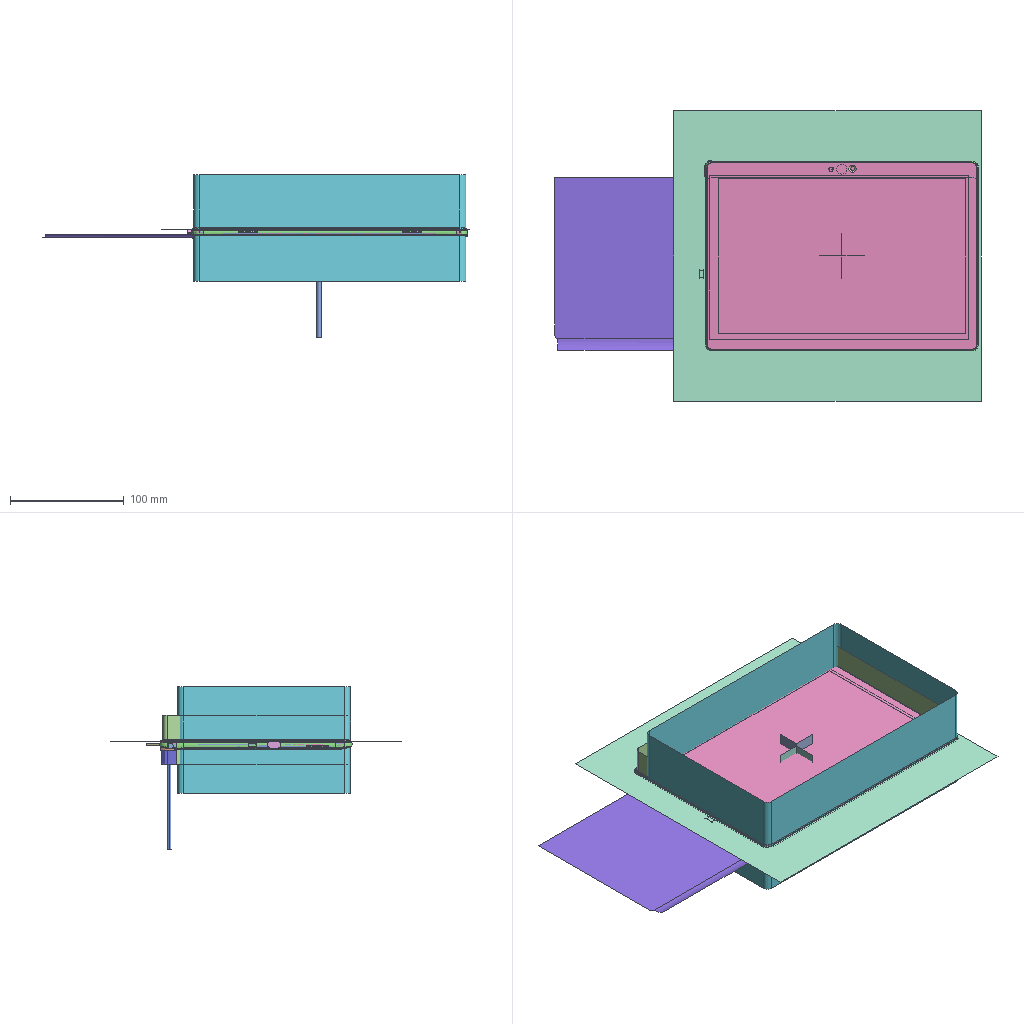Assembly | Creo | 321 different items | 1427 placed | box 375 x 255 x 143 mm
Parts list (item | name | quantity | parent item | size | volume):
1 | - | x1 | in 286 | 3.033 x 2.65 x 3.533 mm | 2.841 mm3
2 | - | x1 | in 314 | 0.2016 x 0.1 x 0.1125 mm | 0.002268 mm3
3 | - | x1 | in 314 | 0.2016 x 0.1 x 0.1125 mm | 0.002268 mm3
4 | - | x1 | in 314 | 0.2016 x 0.1 x 0.1125 mm | 0.002268 mm3
5 | - | x1 | in 314 | 0.2016 x 0.1 x 0.1125 mm | 0.002268 mm3
6 | - | x1 | in 314 | 0.2016 x 0.1 x 0.1125 mm | 0.002268 mm3
7 | - | x1 | in 314 | 0.2016 x 0.1 x 0.1125 mm | 0.002268 mm3
8 | - | x1 | in 314 | 0.2016 x 0.1 x 0.1125 mm | 0.002268 mm3
9 | - | x1 | in 314 | 0.2016 x 0.1 x 0.1125 mm | 0.002268 mm3
10 | - | x1 | in 314 | 0.2016 x 0.1 x 0.1125 mm | 0.002268 mm3
11 | - | x1 | in 314 | 0.2016 x 0.1 x 0.1125 mm | 0.002268 mm3
12 | - | x1 | in 286 | 3.115 x 3.9 x 2.85 mm | 3.729 mm3
13 | - | x14 | in 314 | 1.218 x 0.6006 x 0.55 mm | 0.4024 mm3
14 | - | x1 | in 304 | 0.365 x 0.3 x 0.5 mm | 0.03234 mm3
15 | - | x1 | in 306 | 0.12 x 0.73 x 2.69 mm | 0.132 mm3
16 | - | x1 | in 306 | 0.365 x 0.3 x 0.5 mm | 0.03234 mm3
17 | - | x1 | in 304 | 0.12 x 0.73 x 2.69 mm | 0.132 mm3
18 | - | x1 | in 314 | 1.75 x 2.2 x 1.1 mm | 4.235 mm3
19 | - | x3 | in 314 | 2 x 1.625 x 1.1 mm | 3.576 mm3
20 | - | x1 | in 308 | 42 x 1.4 x 3.75 mm | 72.804 mm3
21 | - | x1 | in 293 | 228.88 x 4.8 x 3.7 mm | 376.003 mm3
22 | - | x1 | in 293 | 8 x 8 x 0.5 mm | 23.747 mm3
23 | - | x1 | in 286 | 3.115 x 3.9 x 2.95 mm | 3.733 mm3
24 | - | x1 | in 303 | 4.45 x 4.45 x 16 mm | 145.448 mm3
25 | - | x1 | in 314 | 3.23 x 3.512 x 0.8 mm | 9.074 mm3
26 | - | x1 | in 313 | 29.01 x 14.6 x 1 mm | 102.876 mm3
27 | - | x1 | in 314 | 14.835 x 14.835 x 0.78 mm | 171.667 mm3
28 | - | x7 | in 314 | 1.64 x 1.15 x 0.5 mm | 0.9427 mm3
29 | - | x1 | in 314 | 14.427 x 18.427 x 1.4 mm | 372.198 mm3
30 | - | x2 | in 314 | 1.95 x 1.55 x 0.6 mm | 1.813 mm3
31 | - | x1 | in 314 | 1.602 x 1.209 x 1.003 mm | 1.943 mm3
32 | - | x1 | in 314 | 7.035 x 7.035 x 0.9 mm | 44.542 mm3
33 | - | x1 | in 314 | 2.45 x 1.685 x 1 mm | 4.128 mm3
34 | - | x1 | in 313 | 7.8 x 3.471 x 1.037 mm | 14.743 mm3
35 | - | x1 | in 287 | 3.6 x 2.85 x 0.98 mm | 3.689 mm3
36 | - | x1 | in 288 | 7.05 x 2.85 x 0.98 mm | 7.612 mm3
37 | - | x1 | in 289 | 6.15 x 2.85 x 0.98 mm | 6.669 mm3
38 | - | x1 | in 288 | 0.9275 x 2.732 x 0.12 mm | 0.1258 mm3
39 | - | x1 | in 289 | 1.038 x 2.73 x 0.12 mm | 0.1282 mm3
40 | - | x1 | in 287 | 3.6 x 1.55 x 0.44 mm | 1.856 mm3
41 | - | x1 | in 288 | 6.83 x 1.56 x 0.4631 mm | 3.381 mm3
42 | - | x1 | in 289 | 5.96 x 1.56 x 0.4431 mm | 2.904 mm3
43 | - | x1 | in 288 | 0.9275 x 2.732 x 0.12 mm | 0.1258 mm3
44 | - | x1 | in 288 | 0.9275 x 2.732 x 0.12 mm | 0.1258 mm3
45 | - | x1 | in 313 | 9 x 7.45 x 3.03 mm | 57.708 mm3
46 | - | x1 | in 289 | 0.9275 x 2.732 x 0.12 mm | 0.1258 mm3
47 | - | x2 | in 287, 288 | 0.9275 x 2.732 x 0.12 mm | 0.1258 mm3
48 | - | x1 | in 289 | 0.9275 x 2.732 x 0.12 mm | 0.1258 mm3
49 | - | x2 | in 287, 288 | 0.9275 x 2.732 x 0.12 mm | 0.1258 mm3
50 | - | x1 | in 289 | 0.9275 x 2.732 x 0.12 mm | 0.1258 mm3
51 | - | x2 | in 287, 288 | 0.9275 x 2.732 x 0.12 mm | 0.1258 mm3
52 | - | x1 | in 289 | 0.9275 x 2.732 x 0.12 mm | 0.1258 mm3
53 | - | x2 | in 287, 288 | 0.9275 x 2.732 x 0.12 mm | 0.1258 mm3
54 | - | x1 | in 289 | 0.9275 x 2.732 x 0.12 mm | 0.1258 mm3
55 | - | x2 | in 287, 288 | 0.9275 x 2.732 x 0.12 mm | 0.1258 mm3
56 | - | x1 | in 305 | 12.79 x 0.475 x 1.585 mm | 6 mm3
57 | - | x1 | in 289 | 0.9275 x 2.732 x 0.12 mm | 0.1258 mm3
58 | - | x2 | in 287, 288 | 0.9275 x 2.732 x 0.12 mm | 0.1258 mm3
59 | - | x1 | in 289 | 0.9275 x 2.732 x 0.12 mm | 0.1258 mm3
60 | - | x1 | in 288 | 0.9275 x 2.732 x 0.12 mm | 0.1258 mm3
61 | - | x1 | in 289 | 0.9275 x 2.732 x 0.12 mm | 0.1258 mm3
62 | - | x1 | in 289 | 0.9275 x 2.732 x 0.12 mm | 0.1258 mm3
63 | - | x1 | in 289 | 1.038 x 2.73 x 0.12 mm | 0.1282 mm3
64 | - | x1 | in 288 | 1.038 x 2.73 x 0.12 mm | 0.1282 mm3
65 | - | x1 | in 289 | 1.038 x 2.73 x 0.12 mm | 0.1282 mm3
66 | - | x1 | in 289 | 1.038 x 2.73 x 0.12 mm | 0.1282 mm3
67 | - | x1 | in 314 | 1.4 x 1.1 x 0.5001 mm | 0.7702 mm3
68 | - | x2 | in 287, 288 | 1.038 x 2.73 x 0.12 mm | 0.1282 mm3
69 | - | x1 | in 289 | 1.038 x 2.73 x 0.12 mm | 0.1282 mm3
70 | - | x2 | in 287, 288 | 1.038 x 2.73 x 0.12 mm | 0.1282 mm3
71 | - | x1 | in 289 | 1.038 x 2.73 x 0.12 mm | 0.1282 mm3
72 | - | x2 | in 287, 288 | 1.038 x 2.73 x 0.12 mm | 0.1282 mm3
73 | - | x1 | in 289 | 1.038 x 2.73 x 0.12 mm | 0.1282 mm3
74 | - | x2 | in 287, 288 | 1.038 x 2.73 x 0.12 mm | 0.1282 mm3
75 | - | x1 | in 289 | 1.038 x 2.73 x 0.12 mm | 0.1282 mm3
76 | - | x2 | in 287, 288 | 1.038 x 2.73 x 0.12 mm | 0.1282 mm3
77 | - | x1 | in 289 | 1.038 x 2.73 x 0.12 mm | 0.1282 mm3
78 | - | x1 | in 314 | 1.5 x 1.5 x 1.061 mm | 2.386 mm3
79 | - | x2 | in 287, 288 | 1.038 x 2.73 x 0.12 mm | 0.1282 mm3
80 | - | x1 | in 288 | 1.038 x 2.73 x 0.12 mm | 0.1282 mm3
81 | - | x1 | in 288 | 1.038 x 2.73 x 0.12 mm | 0.1282 mm3
82 | - | x1 | in 288 | 1.038 x 2.73 x 0.12 mm | 0.1282 mm3
83 | - | x1 | in 288 | 1.038 x 2.73 x 0.12 mm | 0.1282 mm3
84 | - | x1 | in 289 | 0.96 x 2.46 x 0.38 mm | 0.1621 mm3
85 | - | x1 | in 288 | 0.96 x 2.46 x 0.38 mm | 0.1619 mm3
86 | - | x1 | in 292 | 0.01 x 0.3 x 0.8 mm | 0.0024 mm3
87 | - | x1 | in 292 | 0.01 x 0.3 x 0.8 mm | 0.0024 mm3
88 | - | x1 | in 292 | 0.01 x 0.3 x 0.8 mm | 0.0024 mm3
89 | - | x1 | - | - | -
90 | - | x1 | in 291 | 0.01 x 0.3 x 0.8 mm | 0.0024 mm3
91 | - | x1 | in 292 | 0.01 x 0.3 x 0.8 mm | 0.0024 mm3
92 | - | x1 | in 291 | 0.01 x 0.3 x 0.8 mm | 0.0024 mm3
93 | - | x1 | in 290 | 0.01 x 0.3 x 0.8 mm | 0.0024 mm3
94 | - | x1 | in 292 | 0.01 x 0.3 x 0.8 mm | 0.0024 mm3
95 | - | x2 | in 290, 291 | 0.01 x 0.3 x 0.8 mm | 0.0024 mm3
96 | - | x1 | in 292 | 0.01 x 0.3 x 0.8 mm | 0.0024 mm3
97 | - | x2 | in 290, 291 | 0.01 x 0.3 x 0.8 mm | 0.0024 mm3
98 | - | x1 | in 292 | 0.01 x 0.3 x 0.8 mm | 0.0024 mm3
99 | - | x2 | in 290, 291 | 0.01 x 0.3 x 0.8 mm | 0.0024 mm3
100 | - | x2 | in 314 | 1.685 x 1.694 x 0.6 mm | 1.713 mm3
101 | - | x1 | in 292 | 0.01 x 0.3 x 0.8 mm | 0.0024 mm3
102 | - | x2 | in 290, 291 | 0.01 x 0.3 x 0.8 mm | 0.0024 mm3
103 | - | x1 | in 292 | 0.01 x 0.3 x 0.8 mm | 0.0024 mm3
104 | - | x2 | in 290, 291 | 0.01 x 0.3 x 0.8 mm | 0.0024 mm3
105 | - | x1 | in 291 | 0.01 x 0.3 x 0.8 mm | 0.0024 mm3
106 | - | x1 | in 291 | 0.01 x 0.3 x 0.8 mm | 0.0024 mm3
107 | - | x1 | in 291 | 0.01 x 0.3 x 0.8 mm | 0.0024 mm3
108 | - | x1 | in 291 | 0.01 x 0.3 x 0.8 mm | 0.0024 mm3
109 | - | x1 | in 292 | 0.01 x 0.3 x 0.65 mm | 0.00195 mm3
110 | - | x1 | in 292 | 0.01 x 0.3 x 0.65 mm | 0.00195 mm3
111 | - | x1 | in 314 | 4 x 3 x 2.5 mm | 30 mm3
112 | - | x6 | in 314 | 2.3 x 1.1 x 1.275 mm | 3.225 mm3
113 | - | x1 | in 292 | 0.01 x 0.3 x 0.65 mm | 0.00195 mm3
114 | - | x1 | in 291 | 0.01 x 0.3 x 0.65 mm | 0.00195 mm3
115 | - | x1 | in 292 | 0.01 x 0.3 x 0.65 mm | 0.00195 mm3
116 | - | x2 | in 290, 291 | 0.01 x 0.3 x 0.65 mm | 0.00195 mm3
117 | - | x1 | in 292 | 0.01 x 0.3 x 0.65 mm | 0.00195 mm3
118 | - | x2 | in 290, 291 | 0.01 x 0.3 x 0.65 mm | 0.00195 mm3
119 | - | x1 | in 292 | 0.01 x 0.3 x 0.65 mm | 0.00195 mm3
120 | - | x2 | in 290, 291 | 0.01 x 0.3 x 0.65 mm | 0.00195 mm3
121 | - | x1 | in 292 | 0.01 x 0.3 x 0.65 mm | 0.00195 mm3
122 | - | x2 | in 290, 291 | 0.01 x 0.3 x 0.65 mm | 0.00195 mm3
123 | - | x1 | in 308 | 145 x 2.8 x 115 mm | 46690 mm3
124 | - | x1 | in 292 | 0.01 x 0.3 x 0.65 mm | 0.00195 mm3
125 | - | x2 | in 290, 291 | 0.01 x 0.3 x 0.65 mm | 0.00195 mm3
126 | - | x1 | in 291 | 0.01 x 0.3 x 0.65 mm | 0.00195 mm3
127 | - | x1 | in 290 | 0.01 x 0.3 x 0.65 mm | 0.00195 mm3
128 | - | x1 | in 292 | 0.01 x 0.3 x 0.65 mm | 0.00195 mm3
129 | - | x1 | in 291 | 0.01 x 0.3 x 0.65 mm | 0.00195 mm3
130 | - | x1 | in 291 | 0.01 x 0.3 x 0.65 mm | 0.00195 mm3
131 | - | x1 | in 291 | 0.01 x 0.3 x 0.65 mm | 0.00195 mm3
132 | - | x1 | in 292 | 0.01 x 0.3 x 1.15 mm | 0.00345 mm3
133 | - | x1 | in 291 | 0.01 x 0.3 x 1.15 mm | 0.00345 mm3
134 | - | x1 | in 314 | 2 x 1.25 x 1.179 mm | 2.948 mm3
135 | - | x1 | in 314 | 2.1 x 1.25 x 1.222 mm | 3.208 mm3
136 | - | x1 | in 314 | 1.677 x 2.114 x 0.5499 mm | 1.949 mm3
137 | - | x192 | in 314 | 1.016 x 0.508 x 0.568 mm | 0.279 mm3
138 | - | x119 | in 314 | 1.676 x 0.762 x 0.7099 mm | 0.9069 mm3
139 | - | x16 | in 314 | 2.413 x 1.27 x 0.9 mm | 2.758 mm3
140 | - | x1 | in 314 | 3 x 1.7 x 1.724 mm | 8.794 mm3
141 | - | x1 | in 314 | 4 x 2 x 2.236 mm | 17.889 mm3
142 | - | x3 | in 314 | 3 x 1.7 x 1.724 mm | 8.794 mm3
143 | - | x5 | in 314 | 1.889 x 0.9288 x 1.053 mm | 1.848 mm3
144 | - | x1 | in 314 | 1.891 x 0.9288 x 1.053 mm | 1.851 mm3
145 | - | x1 | in 293 | 239.13 x 152.07 x 3.674 mm | 36465 mm3
146 | - | x1 | in 314 | 1.925 x 1.657 x 1.27 mm | 4.052 mm3
147 | - | x1 | in 314 | 6.05 x 5.85 x 0.9 mm | 31.853 mm3
148 | - | x1 | in 314 | 1.616 x 1.219 x 1.012 mm | 1.993 mm3
149 | - | x1 | in 314 | 1.95 x 1.55 x 1.245 mm | 3.764 mm3
150 | - | x4 | in 314 | 1.95 x 1.55 x 0.6 mm | 1.813 mm3
151 | - | x1 | in 314 | 2.318 x 2.344 x 1.2 mm | 6.521 mm3
152 | - | x1 | in 314 | 3.529 x 3.425 x 2.459 mm | 29.726 mm3
153 | - | x1 | in 293 | 211.4 x 12.505 x 3.981 mm | 1559 mm3
154 | - | x1 | in 300 | 17.275 x 28.25 x 2.305 mm | 74.352 mm3
155 | - | x1 | in 313 | 41.9 x 42.2 x 1.8 mm | 390.663 mm3
156 | - | x1 | in 320 | 6.77 x 3.923 x 1 mm | 14.09 mm3
157 | - | x1 | in 313 | 12.1 x 15.71 x 1.8 mm | 53.743 mm3
158 | - | x1 | in 313 | 27.4 x 27.7 x 1.8 mm | 180.699 mm3
159 | - | x1 | in 294 | 29.8 x 40.77 x 0.3 mm | 245.433 mm3
160 | - | x1 | in 314 | 2.368 x 2.475 x 0.6 mm | 3.517 mm3
161 | - | x1 | in 314 | 7.175 x 4.435 x 1 mm | 31.821 mm3
162 | - | x1 | in 314 | 1.6 x 3.567 x 1.955 mm | 11.154 mm3
163 | - | x2 | in 314 | 1.6 x 3.567 x 0.8499 mm | 4.85 mm3
164 | - | x2 | in 314 | 2 x 0.95 x 1.107 mm | 2.103 mm3
165 | - | x1 | in 314 | 3.425 x 3.725 x 0.03048 mm | 0.389 mm3
166 | - | x7 | in 314 | 3.43 x 3.71 x 0.03048 mm | 0.3879 mm3
167 | - | x3 | in 321 | 4.77 x 3.923 x 1 mm | 9.925 mm3
168 | - | x3 | in 314 | 3.127 x 3.363 x 1.25 mm | 13.145 mm3
169 | - | x1 | in 314 | 2.094 x 1.8 x 1.381 mm | 5.204 mm3
170 | - | x1 | in 314 | 2.974 x 2.49 x 1 mm | 7.406 mm3
171 | - | x35 | in 314 | 1.2 x 1.2 x 0.8485 mm | 1.222 mm3
172 | - | x1 | in 314 | 1 x 1 x 0.7071 mm | 0.7071 mm3
173 | - | x1 | in 314 | 1.2 x 1.2 x 0.8485 mm | 1.222 mm3
174 | - | x1 | in 314 | 1.2 x 1.2 x 0.8485 mm | 1.222 mm3
175 | - | x1 | in 314 | 1.2 x 1.2 x 0.8485 mm | 1.222 mm3
176 | - | x1 | in 314 | 1.2 x 1.2 x 0.8485 mm | 1.222 mm3
177 | - | x1 | in 314 | 1 x 1 x 0.2 mm | 0.2 mm3
178 | - | x1 | in 301 | 5.77 x 3.923 x 1 mm | 12.056 mm3
179 | - | x1 | in 314 | 1 x 1 x 0.7071 mm | 0.7071 mm3
180 | - | x1 | in 314 | 1 x 1 x 0.7071 mm | 0.7071 mm3
181 | - | x1 | in 314 | 1 x 1 x 0.7071 mm | 0.7071 mm3
182 | - | x1 | in 314 | 1 x 1 x 0.7071 mm | 0.7071 mm3
183 | - | x1 | in 314 | 1 x 1 x 1 mm | 1 mm3
184 | - | x1 | in 314 | 1 x 1 x 0.7071 mm | 0.7071 mm3
185 | - | x1 | in 314 | 1 x 1 x 0.7071 mm | 0.7071 mm3
186 | - | x1 | in 314 | 1 x 1 x 0.7071 mm | 0.7071 mm3
187 | - | x1 | in 314 | 1 x 1 x 0.7071 mm | 0.7071 mm3
188 | - | x1 | in 314 | 1 x 1 x 0.7071 mm | 0.7071 mm3
189 | - | x323 | in 314 | 1.016 x 0.508 x 0.35 mm | 0.1806 mm3
190 | - | x1 | in 314 | 1 x 1 x 0.7071 mm | 0.7071 mm3
191 | - | x1 | in 314 | 1 x 1 x 0.7071 mm | 0.7071 mm3
192 | - | x1 | in 314 | 1 x 1 x 0.7071 mm | 0.7071 mm3
193 | - | x2 | in 314 | 1 x 1 x 0.7071 mm | 0.7071 mm3
194 | - | x1 | in 285 | 8.29 x 2.815 x 7.15 mm | 54.664 mm3
195 | - | x2 | in 310 | - | -
196 | - | x1 | in 314 | 2.175 x 2.175 x 1.2 mm | 5.677 mm3
197 | - | x1 | in 314 | 2.061 x 2.115 x 1.477 mm | 6.439 mm3
198 | - | x1 | in 314 | 1.91 x 2.31 x 1.499 mm | 6.612 mm3
199 | - | x1 | in 314 | 2.236 x 2.636 x 0.6251 mm | 3.684 mm3
200 | - | x86 | in 314 | 1.676 x 0.762 x 0.55 mm | 0.7026 mm3
201 | - | x1 | in 314 | 5 x 5 x 0.8999 mm | 22.498 mm3
202 | - | x1 | in 293 | 2.96 x 139.6 x 4.9 mm | 378.881 mm3
203 | - | x1 | in 308 | - | 51565 mm3
204 | - | x1 | in 313 | 121 x 59 x 1 mm | 6613 mm3
205 | - | x78 | in 314 | 2.413 x 1.27 x 0.9 mm | 2.758 mm3
206 | - | x2 | in 314 | 1.95 x 1.55 x 0.6 mm | 1.813 mm3
207 | - | x1 | in 314 | 3 x 1.7 x 1.55 mm | 7.906 mm3
208 | - | x20 | in 305 | 0.12 x 0.98 x 2.75 mm | 0.1279 mm3
209 | - | x19 | in 305 | 0.12 x 0.865 x 2.691 mm | 0.1098 mm3
210 | - | x1 | in 295 | 8.5 x 8.45 x 8.5 mm | 356.367 mm3
211 | - | x1 | in 295 | 18.5 x 1.9 x 75.87 mm | 163.267 mm3
212 | - | x1 | in 308 | 8.5 x 9.659 x 8.5 mm | 422.481 mm3
213 | - | x1 | in 314 | 2.614 x 2.213 x 0.5 mm | 2.892 mm3
214 | - | x1 | in 314 | 1.75 x 0.95 x 0.9956 mm | 1.655 mm3
215 | - | x1 | in 314 | 2.272 x 2.272 x 1.606 mm | 8.291 mm3
216 | - | x1 | in 302 | 239.74 x 166.74 x 6.94 mm | 15309 mm3
217 | - | x1 | in 314 | 4 x 3 x 2.25 mm | 27 mm3
218 | - | x1 | in 308 | 10.47 x 4.152 x 65.568 mm | 124.944 mm3
219 | - | x1 | in 308 | - | 52.759 mm3
220 | - | x1 | in 314 | 3.1 x 1.8 x 1.792 mm | 10.001 mm3
221 | - | x1 | in 305 | 13.2 x 0.97 x 2.9 mm | 14.533 mm3
222 | - | x1 | - | - | -
223 | - | x1 | in 314 | 3 x 2.6 x 0.8 mm | 6.24 mm3
224 | - | x112 | in 314 | 1.016 x 0.508 x 0.35 mm | 0.1806 mm3
225 | - | x6 | in 314 | 1.676 x 0.762 x 0.7099 mm | 0.9069 mm3
226 | - | x1 | in 314 | 2.413 x 1.27 x 0.9 mm | 2.758 mm3
227 | - | x1 | in 314 | 3.6 x 3.6 x 1.02 mm | 13.22 mm3
228 | - | x2 | in 314 | 1.107 x 0.6124 x 0.6325 mm | 0.4288 mm3
229 | - | x6 | in 314 | 2.8 x 2.3 x 1.02 mm | 6.569 mm3
230 | - | x11 | in 314 | 2.2 x 1.8 x 0.95 mm | 3.762 mm3
231 | - | x2 | in 308 | 152.07 x 7.3 x 217.3 mm | 28108 mm3
232 | - | x1 | in 307 | 4.8 x 4.6 x 9.4 mm | 182.133 mm3
233 | - | x1 | in 307 | 4.2 x 3.2 x 3 mm | 19.597 mm3
234 | - | x1 | in 320 | 0.15 x 0.7581 x 0.2242 mm | 0.01667 mm3
235 | - | x1 | in 320 | 0.15 x 0.7581 x 0.2242 mm | 0.01667 mm3
236 | - | x1 | in 320 | 0.15 x 0.7581 x 0.2242 mm | 0.01667 mm3
237 | - | x1 | in 320 | 0.15 x 0.7581 x 0.2242 mm | 0.01667 mm3
238 | - | x1 | in 320 | 0.15 x 0.7581 x 0.2242 mm | 0.01667 mm3
239 | - | x1 | in 308 | 228.6 x 13.85 x 143 mm | 73471 mm3
240 | - | x1 | in 320 | 0.15 x 0.7581 x 0.2242 mm | 0.01667 mm3
241 | - | x1 | in 320 | 0.15 x 0.7581 x 0.2242 mm | 0.01667 mm3
242 | - | x3 | in 321 | 0.15 x 0.7581 x 0.2242 mm | 0.01667 mm3
243 | - | x3 | in 321 | 0.15 x 0.7581 x 0.2242 mm | 0.01667 mm3
244 | - | x3 | in 321 | 0.15 x 0.7581 x 0.2242 mm | 0.01667 mm3
245 | - | x3 | in 321 | 0.15 x 0.7581 x 0.2242 mm | 0.01667 mm3
246 | - | x1 | in 320 | 0.15 x 0.7581 x 0.2242 mm | 0.01667 mm3
247 | - | x3 | in 321 | 0.15 x 0.7581 x 0.2242 mm | 0.01667 mm3
248 | - | x3 | in 321 | 0.15 x 0.7581 x 0.2242 mm | 0.01667 mm3
249 | - | x1 | in 320 | 0.15 x 0.7581 x 0.2242 mm | 0.01667 mm3
250 | - | x1 | in 286 | 4.9 x 5.245 x 3.55 mm | 3.146 mm3
251 | - | x1 | in 320 | 0.15 x 0.7581 x 0.2242 mm | 0.01667 mm3
252 | - | x1 | in 301 | 0.15 x 0.7581 x 0.2242 mm | 0.01667 mm3
253 | - | x1 | in 301 | 0.15 x 0.7581 x 0.2242 mm | 0.01667 mm3
254 | - | x1 | in 301 | 0.15 x 0.7581 x 0.2242 mm | 0.01667 mm3
255 | - | x1 | in 301 | 0.15 x 0.7581 x 0.2242 mm | 0.01667 mm3
256 | - | x1 | in 301 | 0.15 x 0.7581 x 0.2242 mm | 0.01667 mm3
257 | - | x1 | in 301 | 0.15 x 0.7581 x 0.2242 mm | 0.01667 mm3
258 | - | x1 | in 301 | 0.15 x 0.7581 x 0.2242 mm | 0.01667 mm3
259 | - | x1 | in 301 | 0.15 x 0.7581 x 0.2242 mm | 0.01667 mm3
260 | - | x1 | in 284 | 8.29 x 2.815 x 7.15 mm | 54.664 mm3
261 | - | x1 | in 286 | 8.3 x 12 x 4.3 mm | 132.29 mm3
262 | - | x1 | in 284 | 11.34 x 5.56 x 6.53 mm | 290.585 mm3
263 | - | x1 | in 314 | 7.5 x 1.55 x 1.5 mm | 17.437 mm3
264 | - | x1 | in 300 | 9.6 x 0.9296 x 8.36 mm | 22.502 mm3
265 | - | x1 | in 293 | 242.355 x 168.94 x 7.8 mm | 215366 mm3
266 | - | x1 | in 314 | 7.835 x 7.835 x 0.8999 mm | 55.244 mm3
267 | - | x1 | in 314 | 4.663 x 4.663 x 0.9 mm | 19.573 mm3
268 | - | x1 | in 314 | 2.02 x 1.72 x 0.8 mm | 2.78 mm3
269 | - | x1 | in 300 | 8.25 x 8 x 0.8796 mm | 10.592 mm3
270 | - | x1 | in 300 | 8.25 x 8 x 0.8796 mm | 10.592 mm3
271 | - | x4 | in 296 | - | -
272 | - | x1 | in 286 | 4.9 x 5.245 x 3.55 mm | 3.175 mm3
273 | - | x2 | in 314 | 0.2032 x 0.1016 x 0.1136 mm | 0.002345 mm3
274 | - | x1 | in 314 | 0.2032 x 0.1016 x 0.1136 mm | 0.002345 mm3
275 | - | x1 | in 314 | 0.2032 x 0.1016 x 0.1136 mm | 0.002345 mm3
276 | - | x1 | in 314 | 0.2016 x 0.1 x 0.1125 mm | 0.002268 mm3
277 | - | x1 | in 314 | 0.2016 x 0.1 x 0.1125 mm | 0.002268 mm3
278 | - | x1 | in 314 | 0.2016 x 0.1 x 0.1125 mm | 0.002268 mm3
279 | - | x1 | in 314 | 0.2016 x 0.1 x 0.1125 mm | 0.002268 mm3
280 | - | x1 | in 314 | 0.2016 x 0.1 x 0.1125 mm | 0.002268 mm3
281 | - | x1 | in 314 | 0.2016 x 0.1 x 0.1125 mm | 0.002268 mm3
282 | - | x1 | in 314 | 0.2016 x 0.1 x 0.1125 mm | 0.002268 mm3
283 | - | x1 | in 313 | - | 114.548 mm3
284 | (subassembly) | x1 | in 313 | - | -
285 | (subassembly) | x1 | in 313 | - | -
286 | (subassembly) | x1 | in 303 | - | -
287 | (subassembly) | x1 | in 318 | - | -
288 | (subassembly) | x1 | in 317 | - | -
289 | (subassembly) | x1 | in 316 | - | -
290 | (subassembly) | x1 | in 287 | - | -
291 | (subassembly) | x1 | in 288 | - | -
292 | (subassembly) | x1 | in 289 | - | -
293 | (subassembly) | x1 | - | - | -
294 | (subassembly) | x1 | in 313 | - | -
295 | (subassembly) | x1 | in 308 | - | -
296 | (subassembly) | x2 | in 310 | - | -
297 | (subassembly) | x1 | in 298 | - | -
298 | (subassembly) | x1 | in 299 | - | -
299 | (subassembly) | x1 | in 313 | - | -
300 | (subassembly) | x1 | in 311 | - | -
301 | (subassembly) | x1 | in 313 | - | -
302 | (subassembly) | x1 | - | - | -
303 | (subassembly) | x1 | in 313 | - | -
304 | (subassembly) | x1 | in 305 | - | -
305 | (subassembly) | x1 | in 309 | - | -
306 | (subassembly) | x1 | in 305 | - | -
307 | (subassembly) | x1 | in 308 | - | -
308 | (subassembly) | x1 | - | - | -
309 | (subassembly) | x1 | in 313 | - | -
310 | (subassembly) | x2 | in 300 | - | -
311 | (subassembly) | x1 | in 294 | - | -
312 | (subassembly) | x1 | in 308 | - | -
313 | (subassembly) | x1 | in 312 | - | -
314 | (subassembly) | x1 | in 315 | - | -
315 | (subassembly) | x1 | in 313 | - | -
316 | (subassembly) | x1 | in 299 | - | -
317 | (subassembly) | x1 | in 297 | - | -
318 | (subassembly) | x1 | in 297 | - | -
319 | (subassembly) | x1 | in 313 | - | -
320 | (subassembly) | x1 | in 319 | - | -
321 | (subassembly) | x3 | in 313 | - | -
Mates (type | each side: item.copy, entity, surface, feature):
In subassembly 308
ASM_CONSTRAINT_MATE_OFF | 216.1 plane datum plane | 203.1 plane datum plane | 2 times
ASM_CONSTRAINT_ALIGN_OFF | 216.1 face plane copy geometry | 203.1 face plane import feature
ASM_CONSTRAINT_INSERT | 203.1 face cylinder surface | 218.1 face cylinder import feature | 2 times
ASM_CONSTRAINT_MATE_OFF | 203.1 face plane import feature | 218.1 face plane import feature
ASM_CONSTRAINT_MATE_OFF | 203.1 face plane surface | 239.1 face plane surface
ASM_CONSTRAINT_MATE | 203.1 face plane surface | 239.1 face plane surface
ASM_CONSTRAINT_MATE_OFF | 203.1 face plane offset | 239.1 face plane import feature
ASM_CONSTRAINT_INSERT | 89.1 face cylinder surface | 20.1 face cylinder import feature
ASM_CONSTRAINT_ALIGN_OFF | 89.1 plane datum plane | 20.1 face plane import feature
ASM_CONSTRAINT_MATE_ANG_OFF | 89.1 plane datum plane | 20.1 face plane surface
ASM_CONSTRAINT_MATE_OFF | 239.1 face plane surface | 231.1 face plane surface
ASM_CONSTRAINT_MATE_OFF | 239.1 face plane import feature | 231.1 face plane import feature | 2 times
ASM_CONSTRAINT_MATE_OFF | 239.1 face plane surface | 231.2 face plane surface
ASM_CONSTRAINT_MATE_OFF | 239.1 face plane import feature | 231.2 face plane import feature | 2 times
ASM_CONSTRAINT_INSERT | 89.1 face cylinder surface | 212.1 face cylinder import feature
ASM_CONSTRAINT_ALIGN_NODEP_ANGLE | 89.1 plane datum plane | 212.1 face plane import feature
ASM_CONSTRAINT_ALIGN_OFF | 89.1 plane datum plane | 212.1 face plane import feature
ASM_CONSTRAINT_INSERT | 203.1 face cylinder cut | 210.1 face cylinder import feature
ASM_CONSTRAINT_ALIGN_OFF | 203.1 face plane import feature | 210.1 face plane import feature
ASM_CONSTRAINT_MATE_ANG_OFF | 203.1 face plane surface | 210.1 face plane import feature
ASM_CONSTRAINT_MATE_OFF | 239.1 face plane import feature | 204.1 face plane import feature
ASM_CONSTRAINT_MATE_OFF | 239.1 face plane surface | 312.1 plane datum plane
ASM_CONSTRAINT_ALIGN_OFF | 239.1 face plane surface | 155.1 face plane import feature
ASM_CONSTRAINT_MATE_OFF | 239.1 face plane import feature | 123.1 face plane protrusion
ASM_CONSTRAINT_MATE_OFF | 218.1 face plane import feature | 219.1 face plane import feature | 3 times
ASM_CONSTRAINT_MATE_OFF | 216.1 face plane protrusion | 232.1 face plane import feature
In subassembly 295
ASM_CONSTRAINT_FIX | assembly other | 2 times
ASM_CONSTRAINT_ALIGN_OFF | 210.2 face plane import feature | 211.1 face plane import feature
In subassembly 307
ASM_CONSTRAINT_ALIGN_OFF | assembly other | 232.2 face plane import feature
ASM_CONSTRAINT_FIX | assembly other | 2 times
ASM_CONSTRAINT_INSERT | 232.2 face cylinder import feature | 233.1 face cylinder import feature